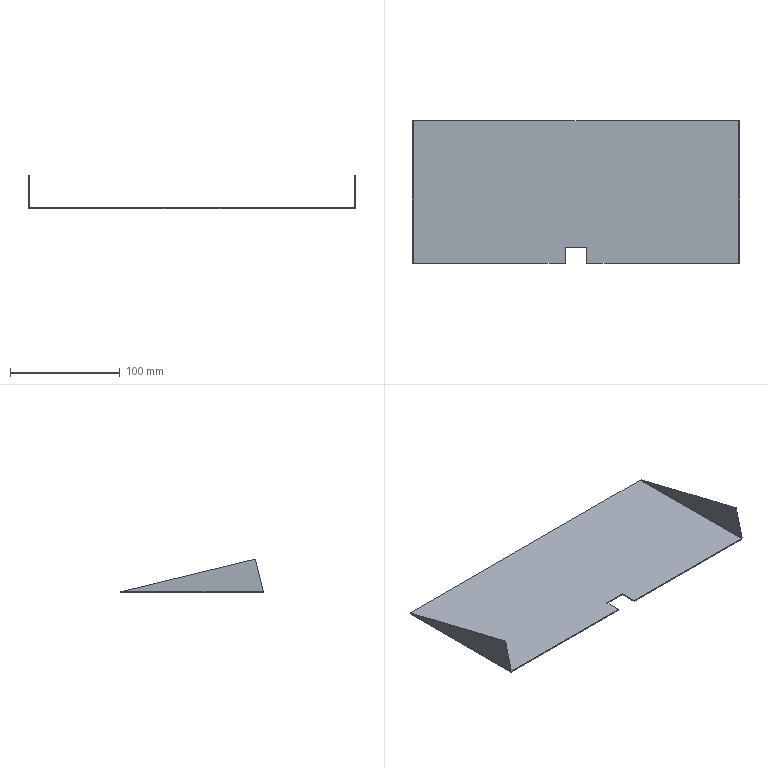Part | SolidWorks | features Cut 1, EdgeFlange 1, FlatPattern 1, MirrorPattern 1, SMBaseFlange 1, SheetMetal 1 | 1 solid | 24 faces | box 299 x 130.5 x 31 mm | volume 42555 mm3 | plane 16 | spline 4 | cylinder 4 | commonest cylinder face diameters 0.4 x2 2.4 x2
STEP:
#1=CARTESIAN_POINT('',(10.,-65.25,-1.));
#2=VERTEX_POINT('',#1);
#3=CARTESIAN_POINT('',(10.,-65.25,0.));
#4=VERTEX_POINT('',#3);
#5=CARTESIAN_POINT('',(10.,-65.25,-1.));
#6=DIRECTION('',(0.,0.,1.));
#7=VECTOR('',#6,1000.);
#8=LINE('',#5,#7);
#9=EDGE_CURVE('',#2,#4,#8,.T.);
#10=ORIENTED_EDGE('',*,*,#9,.F.);
#11=CARTESIAN_POINT('',(148.3,-65.25,-1.));
#12=VERTEX_POINT('',#11);
#13=CARTESIAN_POINT('',(-149.5,-65.25,-1.));
#14=DIRECTION('',(1.,0.,0.));
#15=VECTOR('',#14,1000.);
#16=LINE('',#13,#15);
#17=EDGE_CURVE('',#2,#12,#16,.T.);
#18=ORIENTED_EDGE('',*,*,#17,.T.);
#19=CARTESIAN_POINT('',(148.3,-65.25,0.));
#20=VERTEX_POINT('',#19);
#21=CARTESIAN_POINT('',(148.3,-65.25,0.));
#22=DIRECTION('',(0.,0.,-1.));
#23=VECTOR('',#22,1000.);
#24=LINE('',#21,#23);
#25=EDGE_CURVE('',#20,#12,#24,.T.);
#26=ORIENTED_EDGE('',*,*,#25,.F.);
#27=CARTESIAN_POINT('',(-149.5,-65.25,0.));
#28=DIRECTION('',(1.,0.,0.));
#29=VECTOR('',#28,1000.);
#30=LINE('',#27,#29);
#31=EDGE_CURVE('',#4,#20,#30,.T.);
#32=ORIENTED_EDGE('',*,*,#31,.F.);
#33=EDGE_LOOP('',(#10,#18,#26,#32));
#34=FACE_OUTER_BOUND('',#33,.T.);
#35=CARTESIAN_POINT('',(-149.5,-65.25,-1.));
#36=DIRECTION('',(0.,-1.,0.));
#37=DIRECTION('',(0.,0.,-1.));
#38=AXIS2_PLACEMENT_3D('',#35,#36,#37);
#39=PLANE('',#38);
#40=ADVANCED_FACE('',(#34),#39,.T.);
#41=ORIENTED_EDGE('',*,*,#17,.F.);
#42=CARTESIAN_POINT('',(10.,-50.25,-1.));
#43=VERTEX_POINT('',#42);
#44=CARTESIAN_POINT('',(10.,0.,-1.));
#45=DIRECTION('',(0.,1.,0.));
#46=VECTOR('',#45,1000.);
#47=LINE('',#44,#46);
#48=EDGE_CURVE('',#2,#43,#47,.T.);
#49=ORIENTED_EDGE('',*,*,#48,.T.);
#50=CARTESIAN_POINT('',(-10.,-50.25,-1.));
#51=VERTEX_POINT('',#50);
#52=CARTESIAN_POINT('',(0.,-50.25,-1.));
#53=DIRECTION('',(-1.,0.,0.));
#54=VECTOR('',#53,1000.);
#55=LINE('',#52,#54);
#56=EDGE_CURVE('',#43,#51,#55,.T.);
#57=ORIENTED_EDGE('',*,*,#56,.T.);
#58=CARTESIAN_POINT('',(-10.,-65.25,-1.));
#59=VERTEX_POINT('',#58);
#60=CARTESIAN_POINT('',(-10.,0.,-1.));
#61=DIRECTION('',(0.,-1.,0.));
#62=VECTOR('',#61,1000.);
#63=LINE('',#60,#62);
#64=EDGE_CURVE('',#51,#59,#63,.T.);
#65=ORIENTED_EDGE('',*,*,#64,.T.);
#66=CARTESIAN_POINT('',(-148.3,-65.25,-1.));
#67=VERTEX_POINT('',#66);
#68=CARTESIAN_POINT('',(-149.5,-65.25,-1.));
#69=DIRECTION('',(1.,0.,0.));
#70=VECTOR('',#69,1000.);
#71=LINE('',#68,#70);
#72=EDGE_CURVE('',#67,#59,#71,.T.);
#73=ORIENTED_EDGE('',*,*,#72,.F.);
#74=CARTESIAN_POINT('',(-148.3,65.25,-1.));
#75=VERTEX_POINT('',#74);
#76=CARTESIAN_POINT('',(-148.3,-65.25,-1.));
#77=DIRECTION('',(0.,1.,0.));
#78=VECTOR('',#77,1000.);
#79=LINE('',#76,#78);
#80=EDGE_CURVE('',#67,#75,#79,.T.);
#81=ORIENTED_EDGE('',*,*,#80,.T.);
#82=CARTESIAN_POINT('',(148.3,65.25,-1.));
#83=VERTEX_POINT('',#82);
#84=CARTESIAN_POINT('',(-149.5,65.25,-1.));
#85=DIRECTION('',(-1.,0.,0.));
#86=VECTOR('',#85,1000.);
#87=LINE('',#84,#86);
#88=EDGE_CURVE('',#83,#75,#87,.T.);
#89=ORIENTED_EDGE('',*,*,#88,.F.);
#90=CARTESIAN_POINT('',(148.3,65.25,-1.));
#91=DIRECTION('',(0.,-1.,0.));
#92=VECTOR('',#91,1000.);
#93=LINE('',#90,#92);
#94=EDGE_CURVE('',#83,#12,#93,.T.);
#95=ORIENTED_EDGE('',*,*,#94,.T.);
#96=EDGE_LOOP('',(#41,#49,#57,#65,#73,#81,#89,#95));
#97=FACE_OUTER_BOUND('',#96,.T.);
#98=CARTESIAN_POINT('',(0.,0.,-1.));
#99=DIRECTION('',(0.,0.,1.));
#100=DIRECTION('',(1.,0.,0.));
#101=AXIS2_PLACEMENT_3D('',#98,#99,#100);
#102=PLANE('',#101);
#103=ADVANCED_FACE('',(#97),#102,.F.);
#104=CARTESIAN_POINT('',(10.,-50.25,0.));
#105=VERTEX_POINT('',#104);
#106=CARTESIAN_POINT('',(10.,-50.25,0.));
#107=DIRECTION('',(0.,1.,0.));
#108=VECTOR('',#107,1000.);
#109=LINE('',#106,#108);
#110=EDGE_CURVE('',#4,#105,#109,.T.);
#111=ORIENTED_EDGE('',*,*,#110,.F.);
#112=ORIENTED_EDGE('',*,*,#31,.T.);
#113=CARTESIAN_POINT('',(148.3,65.25,0.));
#114=VERTEX_POINT('',#113);
#115=CARTESIAN_POINT('',(148.3,65.25,0.));
#116=DIRECTION('',(0.,-1.,0.));
#117=VECTOR('',#116,1000.);
#118=LINE('',#115,#117);
#119=EDGE_CURVE('',#114,#20,#118,.T.);
#120=ORIENTED_EDGE('',*,*,#119,.F.);
#121=CARTESIAN_POINT('',(-148.3,65.25,0.));
#122=VERTEX_POINT('',#121);
#123=CARTESIAN_POINT('',(-149.5,65.25,0.));
#124=DIRECTION('',(-1.,0.,0.));
#125=VECTOR('',#124,1000.);
#126=LINE('',#123,#125);
#127=EDGE_CURVE('',#114,#122,#126,.T.);
#128=ORIENTED_EDGE('',*,*,#127,.T.);
#129=CARTESIAN_POINT('',(-148.3,-65.25,0.));
#130=VERTEX_POINT('',#129);
#131=CARTESIAN_POINT('',(-148.3,-65.25,0.));
#132=DIRECTION('',(0.,1.,0.));
#133=VECTOR('',#132,1000.);
#134=LINE('',#131,#133);
#135=EDGE_CURVE('',#130,#122,#134,.T.);
#136=ORIENTED_EDGE('',*,*,#135,.F.);
#137=CARTESIAN_POINT('',(-10.,-65.25,0.));
#138=VERTEX_POINT('',#137);
#139=CARTESIAN_POINT('',(-149.5,-65.25,0.));
#140=DIRECTION('',(1.,0.,0.));
#141=VECTOR('',#140,1000.);
#142=LINE('',#139,#141);
#143=EDGE_CURVE('',#130,#138,#142,.T.);
#144=ORIENTED_EDGE('',*,*,#143,.T.);
#145=CARTESIAN_POINT('',(-10.,-50.25,0.));
#146=VERTEX_POINT('',#145);
#147=CARTESIAN_POINT('',(-10.,-50.25,0.));
#148=DIRECTION('',(0.,-1.,0.));
#149=VECTOR('',#148,1000.);
#150=LINE('',#147,#149);
#151=EDGE_CURVE('',#146,#138,#150,.T.);
#152=ORIENTED_EDGE('',*,*,#151,.F.);
#153=CARTESIAN_POINT('',(-10.,-50.25,0.));
#154=DIRECTION('',(-1.,0.,0.));
#155=VECTOR('',#154,1000.);
#156=LINE('',#153,#155);
#157=EDGE_CURVE('',#105,#146,#156,.T.);
#158=ORIENTED_EDGE('',*,*,#157,.F.);
#159=EDGE_LOOP('',(#111,#112,#120,#128,#136,#144,#152,#158));
#160=FACE_OUTER_BOUND('',#159,.T.);
#161=CARTESIAN_POINT('',(0.,0.,0.));
#162=DIRECTION('',(0.,0.,1.));
#163=DIRECTION('',(1.,0.,0.));
#164=AXIS2_PLACEMENT_3D('',#161,#162,#163);
#165=PLANE('',#164);
#166=ADVANCED_FACE('',(#160),#165,.T.);
#167=ORIENTED_EDGE('',*,*,#127,.F.);
#168=CARTESIAN_POINT('',(148.3,65.25,0.));
#169=DIRECTION('',(0.,0.,-1.));
#170=VECTOR('',#169,1000.);
#171=LINE('',#168,#170);
#172=EDGE_CURVE('',#114,#83,#171,.T.);
#173=ORIENTED_EDGE('',*,*,#172,.T.);
#174=ORIENTED_EDGE('',*,*,#88,.T.);
#175=CARTESIAN_POINT('',(-148.3,65.25,0.));
#176=DIRECTION('',(0.,0.,-1.));
#177=VECTOR('',#176,1000.);
#178=LINE('',#175,#177);
#179=EDGE_CURVE('',#122,#75,#178,.T.);
#180=ORIENTED_EDGE('',*,*,#179,.F.);
#181=EDGE_LOOP('',(#167,#173,#174,#180));
#182=FACE_OUTER_BOUND('',#181,.T.);
#183=CARTESIAN_POINT('',(-149.5,65.25,-1.));
#184=DIRECTION('',(0.,1.,0.));
#185=DIRECTION('',(0.,0.,1.));
#186=AXIS2_PLACEMENT_3D('',#183,#184,#185);
#187=PLANE('',#186);
#188=ADVANCED_FACE('',(#182),#187,.T.);
#189=CARTESIAN_POINT('',(-10.,-65.25,-1.));
#190=DIRECTION('',(0.,0.,-1.));
#191=VECTOR('',#190,1000.);
#192=LINE('',#189,#191);
#193=EDGE_CURVE('',#138,#59,#192,.T.);
#194=ORIENTED_EDGE('',*,*,#193,.F.);
#195=ORIENTED_EDGE('',*,*,#143,.F.);
#196=CARTESIAN_POINT('',(-148.3,-65.25,0.));
#197=DIRECTION('',(0.,0.,-1.));
#198=VECTOR('',#197,1000.);
#199=LINE('',#196,#198);
#200=EDGE_CURVE('',#130,#67,#199,.T.);
#201=ORIENTED_EDGE('',*,*,#200,.T.);
#202=ORIENTED_EDGE('',*,*,#72,.T.);
#203=EDGE_LOOP('',(#194,#195,#201,#202));
#204=FACE_OUTER_BOUND('',#203,.T.);
#205=CARTESIAN_POINT('',(-149.5,-65.25,-1.));
#206=DIRECTION('',(0.,-1.,0.));
#207=DIRECTION('',(0.,0.,-1.));
#208=AXIS2_PLACEMENT_3D('',#205,#206,#207);
#209=PLANE('',#208);
#210=ADVANCED_FACE('',(#204),#209,.T.);
#211=CARTESIAN_POINT('',(-148.5,64.429,0.2));
#212=VERTEX_POINT('',#211);
#213=CARTESIAN_POINT('',(-149.5,64.429,0.2));
#214=VERTEX_POINT('',#213);
#215=CARTESIAN_POINT('',(-149.5,64.429,0.2));
#216=DIRECTION('',(-1.,0.,0.));
#217=VECTOR('',#216,1000.);
#218=LINE('',#215,#217);
#219=EDGE_CURVE('',#212,#214,#218,.T.);
#220=ORIENTED_EDGE('',*,*,#219,.F.);
#221=CARTESIAN_POINT('',(-148.3,65.25,0.));
#222=CARTESIAN_POINT('',(-148.352,65.113,0.));
#223=CARTESIAN_POINT('',(-148.404,64.976,0.02155));
#224=CARTESIAN_POINT('',(-148.478,64.702,0.0956));
#225=CARTESIAN_POINT('',(-148.5,64.566,0.1476));
#226=CARTESIAN_POINT('',(-148.5,64.429,0.2));
#227=B_SPLINE_CURVE_WITH_KNOTS('',3,(#221,#222,#223,#224,#225,#226),.UNSPECIFIED.,.F.,.F.,(4,2,4),(0.,0.5,1.),.UNSPECIFIED.);
#228=EDGE_CURVE('',#122,#212,#227,.T.);
#229=ORIENTED_EDGE('',*,*,#228,.F.);
#230=ORIENTED_EDGE('',*,*,#179,.T.);
#231=CARTESIAN_POINT('',(-148.3,65.25,-1.));
#232=CARTESIAN_POINT('',(-148.459,65.181,-1.));
#233=CARTESIAN_POINT('',(-148.612,65.114,-0.9695));
#234=CARTESIAN_POINT('',(-148.905,64.976,-0.8483));
#235=CARTESIAN_POINT('',(-149.036,64.908,-0.7606));
#236=CARTESIAN_POINT('',(-149.26,64.771,-0.5372));
#237=CARTESIAN_POINT('',(-149.348,64.703,-0.4051));
#238=CARTESIAN_POINT('',(-149.469,64.566,-0.1141));
#239=CARTESIAN_POINT('',(-149.5,64.498,0.04143));
#240=CARTESIAN_POINT('',(-149.5,64.429,0.2));
#241=B_SPLINE_CURVE_WITH_KNOTS('',3,(#231,#232,#233,#234,#235,#236,#237,#238,#239,#240),.UNSPECIFIED.,.F.,.F.,(4,2,2,2,4),(0.,0.0005105,0.001021,0.001532,0.002042),.UNSPECIFIED.);
#242=EDGE_CURVE('',#75,#214,#241,.T.);
#243=ORIENTED_EDGE('',*,*,#242,.T.);
#244=EDGE_LOOP('',(#220,#229,#230,#243));
#245=FACE_OUTER_BOUND('',#244,.T.);
#246=CARTESIAN_POINT('',(-148.3,65.25,-1.01));
#247=CARTESIAN_POINT('',(-148.458,65.182,-1.01));
#248=CARTESIAN_POINT('',(-148.617,65.113,-0.9785));
#249=CARTESIAN_POINT('',(-148.909,64.976,-0.8573));
#250=CARTESIAN_POINT('',(-149.044,64.908,-0.7676));
#251=CARTESIAN_POINT('',(-149.268,64.771,-0.5436));
#252=CARTESIAN_POINT('',(-149.357,64.702,-0.4094));
#253=CARTESIAN_POINT('',(-149.479,64.566,-0.1167));
#254=CARTESIAN_POINT('',(-149.51,64.497,0.04159));
#255=CARTESIAN_POINT('',(-149.51,64.429,0.2));
#256=CARTESIAN_POINT('',(-148.3,65.25,-1.));
#257=CARTESIAN_POINT('',(-148.457,65.182,-1.));
#258=CARTESIAN_POINT('',(-148.614,65.113,-0.9688));
#259=CARTESIAN_POINT('',(-148.904,64.976,-0.8485));
#260=CARTESIAN_POINT('',(-149.037,64.908,-0.7596));
#261=CARTESIAN_POINT('',(-149.26,64.771,-0.5375));
#262=CARTESIAN_POINT('',(-149.349,64.702,-0.4043));
#263=CARTESIAN_POINT('',(-149.469,64.566,-0.1141));
#264=CARTESIAN_POINT('',(-149.5,64.497,0.0429));
#265=CARTESIAN_POINT('',(-149.5,64.429,0.2));
#266=CARTESIAN_POINT('',(-148.3,65.25,0.));
#267=CARTESIAN_POINT('',(-148.326,65.182,0.));
#268=CARTESIAN_POINT('',(-148.352,65.113,0.005205));
#269=CARTESIAN_POINT('',(-148.401,64.976,0.02524));
#270=CARTESIAN_POINT('',(-148.423,64.908,0.04007));
#271=CARTESIAN_POINT('',(-148.46,64.771,0.07709));
#272=CARTESIAN_POINT('',(-148.475,64.702,0.09928));
#273=CARTESIAN_POINT('',(-148.495,64.566,0.1477));
#274=CARTESIAN_POINT('',(-148.5,64.497,0.1738));
#275=CARTESIAN_POINT('',(-148.5,64.429,0.2));
#276=CARTESIAN_POINT('',(-148.3,65.25,0.0101));
#277=CARTESIAN_POINT('',(-148.325,65.182,0.0101));
#278=CARTESIAN_POINT('',(-148.35,65.113,0.01504));
#279=CARTESIAN_POINT('',(-148.396,64.976,0.03407));
#280=CARTESIAN_POINT('',(-148.417,64.908,0.04814));
#281=CARTESIAN_POINT('',(-148.452,64.771,0.0833));
#282=CARTESIAN_POINT('',(-148.466,64.702,0.1044));
#283=CARTESIAN_POINT('',(-148.485,64.566,0.1503));
#284=CARTESIAN_POINT('',(-148.49,64.497,0.1751));
#285=CARTESIAN_POINT('',(-148.49,64.429,0.2));
#286=B_SPLINE_SURFACE_WITH_KNOTS('',1,3,((#246,#247,#248,#249,#250,#251,#252,#253,#254,#255),(#256,#257,#258,#259,#260,#261,#262,#263,#264,#265),(#266,#267,#268,#269,#270,#271,#272,#273,#274,#275),(#276,#277,#278,#279,#280,#281,#282,#283,#284,#285)),.UNSPECIFIED.,.F.,.F.,.F.,(2,1,1,2),(4,2,2,2,4),(-0.01,0.,1.,1.01),(0.,0.25,0.5,0.75,1.),.UNSPECIFIED.);
#287=ADVANCED_FACE('',(#245),#286,.F.);
#288=CARTESIAN_POINT('',(-148.5,-65.201,0.2));
#289=VERTEX_POINT('',#288);
#290=CARTESIAN_POINT('',(-148.5,-65.201,0.2));
#291=CARTESIAN_POINT('',(-148.5,-65.209,0.1476));
#292=CARTESIAN_POINT('',(-148.478,-65.218,0.0956));
#293=CARTESIAN_POINT('',(-148.404,-65.234,0.02155));
#294=CARTESIAN_POINT('',(-148.352,-65.242,0.));
#295=CARTESIAN_POINT('',(-148.3,-65.25,0.));
#296=B_SPLINE_CURVE_WITH_KNOTS('',3,(#290,#291,#292,#293,#294,#295),.UNSPECIFIED.,.F.,.F.,(4,2,4),(0.,0.5,1.),.UNSPECIFIED.);
#297=EDGE_CURVE('',#289,#130,#296,.T.);
#298=ORIENTED_EDGE('',*,*,#297,.F.);
#299=CARTESIAN_POINT('',(-149.5,-65.201,0.2));
#300=VERTEX_POINT('',#299);
#301=CARTESIAN_POINT('',(-148.5,-65.201,0.2));
#302=DIRECTION('',(-1.,0.,0.));
#303=VECTOR('',#302,1000.);
#304=LINE('',#301,#303);
#305=EDGE_CURVE('',#289,#300,#304,.T.);
#306=ORIENTED_EDGE('',*,*,#305,.T.);
#307=CARTESIAN_POINT('',(-149.5,-65.201,0.2));
#308=CARTESIAN_POINT('',(-149.5,-65.205,0.04292));
#309=CARTESIAN_POINT('',(-149.469,-65.209,-0.1141));
#310=CARTESIAN_POINT('',(-149.349,-65.218,-0.4043));
#311=CARTESIAN_POINT('',(-149.26,-65.222,-0.5375));
#312=CARTESIAN_POINT('',(-149.037,-65.23,-0.7596));
#313=CARTESIAN_POINT('',(-148.904,-65.234,-0.8485));
#314=CARTESIAN_POINT('',(-148.614,-65.242,-0.9688));
#315=CARTESIAN_POINT('',(-148.457,-65.246,-1.));
#316=CARTESIAN_POINT('',(-148.3,-65.25,-1.));
#317=B_SPLINE_CURVE_WITH_KNOTS('',3,(#307,#308,#309,#310,#311,#312,#313,#314,#315,#316),.UNSPECIFIED.,.F.,.F.,(4,2,2,2,4),(0.,0.25,0.5,0.75,1.),.UNSPECIFIED.);
#318=EDGE_CURVE('',#300,#67,#317,.T.);
#319=ORIENTED_EDGE('',*,*,#318,.T.);
#320=ORIENTED_EDGE('',*,*,#200,.F.);
#321=EDGE_LOOP('',(#298,#306,#319,#320));
#322=FACE_OUTER_BOUND('',#321,.T.);
#323=CARTESIAN_POINT('',(-149.51,-65.201,0.2));
#324=CARTESIAN_POINT('',(-149.51,-65.205,0.04158));
#325=CARTESIAN_POINT('',(-149.479,-65.209,-0.1167));
#326=CARTESIAN_POINT('',(-149.357,-65.218,-0.4094));
#327=CARTESIAN_POINT('',(-149.268,-65.222,-0.5436));
#328=CARTESIAN_POINT('',(-149.044,-65.23,-0.7676));
#329=CARTESIAN_POINT('',(-148.909,-65.234,-0.8573));
#330=CARTESIAN_POINT('',(-148.617,-65.242,-0.9785));
#331=CARTESIAN_POINT('',(-148.458,-65.246,-1.01));
#332=CARTESIAN_POINT('',(-148.3,-65.25,-1.01));
#333=CARTESIAN_POINT('',(-149.5,-65.201,0.2));
#334=CARTESIAN_POINT('',(-149.5,-65.205,0.04289));
#335=CARTESIAN_POINT('',(-149.469,-65.209,-0.1141));
#336=CARTESIAN_POINT('',(-149.349,-65.218,-0.4043));
#337=CARTESIAN_POINT('',(-149.26,-65.222,-0.5375));
#338=CARTESIAN_POINT('',(-149.037,-65.23,-0.7596));
#339=CARTESIAN_POINT('',(-148.904,-65.234,-0.8485));
#340=CARTESIAN_POINT('',(-148.614,-65.242,-0.9688));
#341=CARTESIAN_POINT('',(-148.457,-65.246,-1.));
#342=CARTESIAN_POINT('',(-148.3,-65.25,-1.));
#343=CARTESIAN_POINT('',(-148.5,-65.201,0.2));
#344=CARTESIAN_POINT('',(-148.5,-65.205,0.1738));
#345=CARTESIAN_POINT('',(-148.495,-65.209,0.1477));
#346=CARTESIAN_POINT('',(-148.475,-65.218,0.09928));
#347=CARTESIAN_POINT('',(-148.46,-65.222,0.07709));
#348=CARTESIAN_POINT('',(-148.423,-65.23,0.04007));
#349=CARTESIAN_POINT('',(-148.401,-65.234,0.02524));
#350=CARTESIAN_POINT('',(-148.352,-65.242,0.005205));
#351=CARTESIAN_POINT('',(-148.326,-65.246,0.));
#352=CARTESIAN_POINT('',(-148.3,-65.25,0.));
#353=CARTESIAN_POINT('',(-148.49,-65.201,0.2));
#354=CARTESIAN_POINT('',(-148.49,-65.205,0.1751));
#355=CARTESIAN_POINT('',(-148.485,-65.209,0.1503));
#356=CARTESIAN_POINT('',(-148.466,-65.218,0.1044));
#357=CARTESIAN_POINT('',(-148.452,-65.222,0.0833));
#358=CARTESIAN_POINT('',(-148.417,-65.23,0.04814));
#359=CARTESIAN_POINT('',(-148.396,-65.234,0.03407));
#360=CARTESIAN_POINT('',(-148.35,-65.242,0.01504));
#361=CARTESIAN_POINT('',(-148.325,-65.246,0.0101));
#362=CARTESIAN_POINT('',(-148.3,-65.25,0.0101));
#363=B_SPLINE_SURFACE_WITH_KNOTS('',1,3,((#323,#324,#325,#326,#327,#328,#329,#330,#331,#332),(#333,#334,#335,#336,#337,#338,#339,#340,#341,#342),(#343,#344,#345,#346,#347,#348,#349,#350,#351,#352),(#353,#354,#355,#356,#357,#358,#359,#360,#361,#362)),.UNSPECIFIED.,.F.,.F.,.F.,(2,1,1,2),(4,2,2,2,4),(-0.01,0.,1.,1.01),(0.,0.25,0.5,0.75,1.),.UNSPECIFIED.);
#364=ADVANCED_FACE('',(#322),#363,.F.);
#365=ORIENTED_EDGE('',*,*,#80,.F.);
#366=ORIENTED_EDGE('',*,*,#318,.F.);
#367=CARTESIAN_POINT('',(-149.5,64.429,0.2));
#368=DIRECTION('',(0.,1.,0.));
#369=VECTOR('',#368,1000.);
#370=LINE('',#367,#369);
#371=EDGE_CURVE('',#300,#214,#370,.T.);
#372=ORIENTED_EDGE('',*,*,#371,.T.);
#373=ORIENTED_EDGE('',*,*,#242,.F.);
#374=EDGE_LOOP('',(#365,#366,#372,#373));
#375=FACE_OUTER_BOUND('',#374,.T.);
#376=CARTESIAN_POINT('',(-148.3,-65.25,0.2));
#377=DIRECTION('',(0.,-1.,0.));
#378=DIRECTION('',(-1.,0.,0.));
#379=AXIS2_PLACEMENT_3D('',#376,#377,#378);
#380=CYLINDRICAL_SURFACE('',#379,1.2);
#381=ADVANCED_FACE('',(#375),#380,.T.);
#382=ORIENTED_EDGE('',*,*,#135,.T.);
#383=ORIENTED_EDGE('',*,*,#228,.T.);
#384=CARTESIAN_POINT('',(-148.5,64.429,0.2));
#385=DIRECTION('',(0.,-1.,0.));
#386=VECTOR('',#385,1000.);
#387=LINE('',#384,#386);
#388=EDGE_CURVE('',#212,#289,#387,.T.);
#389=ORIENTED_EDGE('',*,*,#388,.T.);
#390=ORIENTED_EDGE('',*,*,#297,.T.);
#391=EDGE_LOOP('',(#382,#383,#389,#390));
#392=FACE_OUTER_BOUND('',#391,.T.);
#393=CARTESIAN_POINT('',(-148.3,-65.25,0.2));
#394=DIRECTION('',(0.,-1.,0.));
#395=DIRECTION('',(-1.,0.,0.));
#396=AXIS2_PLACEMENT_3D('',#393,#394,#395);
#397=CYLINDRICAL_SURFACE('',#396,0.2);
#398=ADVANCED_FACE('',(#392),#397,.F.);
#399=ORIENTED_EDGE('',*,*,#219,.T.);
#400=CARTESIAN_POINT('',(-149.5,-57.944,30.));
#401=VERTEX_POINT('',#400);
#402=CARTESIAN_POINT('',(-149.5,3.653,15.));
#403=DIRECTION('',(0.,0.9716,-0.2366));
#404=VECTOR('',#403,1000.);
#405=LINE('',#402,#404);
#406=EDGE_CURVE('',#401,#214,#405,.T.);
#407=ORIENTED_EDGE('',*,*,#406,.F.);
#408=CARTESIAN_POINT('',(-148.5,-57.944,30.));
#409=VERTEX_POINT('',#408);
#410=CARTESIAN_POINT('',(-149.5,-57.944,30.));
#411=DIRECTION('',(1.,0.,0.));
#412=VECTOR('',#411,1000.);
#413=LINE('',#410,#412);
#414=EDGE_CURVE('',#401,#409,#413,.T.);
#415=ORIENTED_EDGE('',*,*,#414,.T.);
#416=CARTESIAN_POINT('',(-148.5,-57.944,30.));
#417=DIRECTION('',(0.,0.9716,-0.2366));
#418=VECTOR('',#417,1000.);
#419=LINE('',#416,#418);
#420=EDGE_CURVE('',#409,#212,#419,.T.);
#421=ORIENTED_EDGE('',*,*,#420,.T.);
#422=EDGE_LOOP('',(#399,#407,#415,#421));
#423=FACE_OUTER_BOUND('',#422,.T.);
#424=CARTESIAN_POINT('',(-149.5,-57.944,30.));
#425=DIRECTION('',(0.,-0.2366,-0.9716));
#426=DIRECTION('',(0.,0.9716,-0.2366));
#427=AXIS2_PLACEMENT_3D('',#424,#425,#426);
#428=PLANE('',#427);
#429=ADVANCED_FACE('',(#423),#428,.F.);
#430=ORIENTED_EDGE('',*,*,#305,.F.);
#431=CARTESIAN_POINT('',(-148.5,-65.25,0.));
#432=DIRECTION('',(0.,0.2366,0.9716));
#433=VECTOR('',#432,1000.);
#434=LINE('',#431,#433);
#435=EDGE_CURVE('',#289,#409,#434,.T.);
#436=ORIENTED_EDGE('',*,*,#435,.T.);
#437=ORIENTED_EDGE('',*,*,#414,.F.);
#438=CARTESIAN_POINT('',(-149.5,-61.597,15.));
#439=DIRECTION('',(0.,0.2366,0.9716));
#440=VECTOR('',#439,1000.);
#441=LINE('',#438,#440);
#442=EDGE_CURVE('',#300,#401,#441,.T.);
#443=ORIENTED_EDGE('',*,*,#442,.F.);
#444=EDGE_LOOP('',(#430,#436,#437,#443));
#445=FACE_OUTER_BOUND('',#444,.T.);
#446=CARTESIAN_POINT('',(-149.5,-65.25,0.));
#447=DIRECTION('',(0.,0.9716,-0.2366));
#448=DIRECTION('',(0.,0.2366,0.9716));
#449=AXIS2_PLACEMENT_3D('',#446,#447,#448);
#450=PLANE('',#449);
#451=ADVANCED_FACE('',(#445),#450,.F.);
#452=ORIENTED_EDGE('',*,*,#371,.F.);
#453=ORIENTED_EDGE('',*,*,#442,.T.);
#454=ORIENTED_EDGE('',*,*,#406,.T.);
#455=EDGE_LOOP('',(#452,#453,#454));
#456=FACE_OUTER_BOUND('',#455,.T.);
#457=CARTESIAN_POINT('',(-149.5,0.,0.));
#458=DIRECTION('',(1.,0.,0.));
#459=DIRECTION('',(0.,0.,-1.));
#460=AXIS2_PLACEMENT_3D('',#457,#458,#459);
#461=PLANE('',#460);
#462=ADVANCED_FACE('',(#456),#461,.F.);
#463=ORIENTED_EDGE('',*,*,#435,.F.);
#464=ORIENTED_EDGE('',*,*,#388,.F.);
#465=ORIENTED_EDGE('',*,*,#420,.F.);
#466=EDGE_LOOP('',(#463,#464,#465));
#467=FACE_OUTER_BOUND('',#466,.T.);
#468=CARTESIAN_POINT('',(-148.5,0.,0.));
#469=DIRECTION('',(1.,0.,0.));
#470=DIRECTION('',(0.,0.,-1.));
#471=AXIS2_PLACEMENT_3D('',#468,#469,#470);
#472=PLANE('',#471);
#473=ADVANCED_FACE('',(#467),#472,.T.);
#474=CARTESIAN_POINT('',(148.5,-65.201,0.2));
#475=VERTEX_POINT('',#474);
#476=CARTESIAN_POINT('',(149.5,-65.201,0.2));
#477=VERTEX_POINT('',#476);
#478=CARTESIAN_POINT('',(149.5,-65.201,0.2));
#479=DIRECTION('',(1.,0.,0.));
#480=VECTOR('',#479,1000.);
#481=LINE('',#478,#480);
#482=EDGE_CURVE('',#475,#477,#481,.T.);
#483=ORIENTED_EDGE('',*,*,#482,.F.);
#484=CARTESIAN_POINT('',(148.3,-65.25,0.));
#485=CARTESIAN_POINT('',(148.352,-65.242,0.));
#486=CARTESIAN_POINT('',(148.404,-65.234,0.02155));
#487=CARTESIAN_POINT('',(148.478,-65.218,0.0956));
#488=CARTESIAN_POINT('',(148.5,-65.209,0.1476));
#489=CARTESIAN_POINT('',(148.5,-65.201,0.2));
#490=B_SPLINE_CURVE_WITH_KNOTS('',3,(#484,#485,#486,#487,#488,#489),.UNSPECIFIED.,.F.,.F.,(4,2,4),(0.,0.5,1.),.UNSPECIFIED.);
#491=EDGE_CURVE('',#20,#475,#490,.T.);
#492=ORIENTED_EDGE('',*,*,#491,.F.);
#493=ORIENTED_EDGE('',*,*,#25,.T.);
#494=CARTESIAN_POINT('',(148.3,-65.25,-1.));
#495=CARTESIAN_POINT('',(148.457,-65.246,-1.));
#496=CARTESIAN_POINT('',(148.614,-65.242,-0.9688));
#497=CARTESIAN_POINT('',(148.904,-65.234,-0.8485));
#498=CARTESIAN_POINT('',(149.037,-65.23,-0.7596));
#499=CARTESIAN_POINT('',(149.26,-65.222,-0.5375));
#500=CARTESIAN_POINT('',(149.349,-65.218,-0.4043));
#501=CARTESIAN_POINT('',(149.469,-65.209,-0.1141));
#502=CARTESIAN_POINT('',(149.5,-65.205,0.04292));
#503=CARTESIAN_POINT('',(149.5,-65.201,0.2));
#504=B_SPLINE_CURVE_WITH_KNOTS('',3,(#494,#495,#496,#497,#498,#499,#500,#501,#502,#503),.UNSPECIFIED.,.F.,.F.,(4,2,2,2,4),(0.,0.25,0.5,0.75,1.),.UNSPECIFIED.);
#505=EDGE_CURVE('',#12,#477,#504,.T.);
#506=ORIENTED_EDGE('',*,*,#505,.T.);
#507=EDGE_LOOP('',(#483,#492,#493,#506));
#508=FACE_OUTER_BOUND('',#507,.T.);
#509=CARTESIAN_POINT('',(148.3,-65.25,-1.01));
#510=CARTESIAN_POINT('',(148.458,-65.246,-1.01));
#511=CARTESIAN_POINT('',(148.617,-65.242,-0.9785));
#512=CARTESIAN_POINT('',(148.909,-65.234,-0.8573));
#513=CARTESIAN_POINT('',(149.044,-65.23,-0.7676));
#514=CARTESIAN_POINT('',(149.268,-65.222,-0.5436));
#515=CARTESIAN_POINT('',(149.357,-65.218,-0.4094));
#516=CARTESIAN_POINT('',(149.479,-65.209,-0.1167));
#517=CARTESIAN_POINT('',(149.51,-65.205,0.04158));
#518=CARTESIAN_POINT('',(149.51,-65.201,0.2));
#519=CARTESIAN_POINT('',(148.3,-65.25,-1.));
#520=CARTESIAN_POINT('',(148.457,-65.246,-1.));
#521=CARTESIAN_POINT('',(148.614,-65.242,-0.9688));
#522=CARTESIAN_POINT('',(148.904,-65.234,-0.8485));
#523=CARTESIAN_POINT('',(149.037,-65.23,-0.7596));
#524=CARTESIAN_POINT('',(149.26,-65.222,-0.5375));
#525=CARTESIAN_POINT('',(149.349,-65.218,-0.4043));
#526=CARTESIAN_POINT('',(149.469,-65.209,-0.1141));
#527=CARTESIAN_POINT('',(149.5,-65.205,0.04289));
#528=CARTESIAN_POINT('',(149.5,-65.201,0.2));
#529=CARTESIAN_POINT('',(148.3,-65.25,0.));
#530=CARTESIAN_POINT('',(148.326,-65.246,0.));
#531=CARTESIAN_POINT('',(148.352,-65.242,0.005205));
#532=CARTESIAN_POINT('',(148.401,-65.234,0.02524));
#533=CARTESIAN_POINT('',(148.423,-65.23,0.04007));
#534=CARTESIAN_POINT('',(148.46,-65.222,0.07709));
#535=CARTESIAN_POINT('',(148.475,-65.218,0.09928));
#536=CARTESIAN_POINT('',(148.495,-65.209,0.1477));
#537=CARTESIAN_POINT('',(148.5,-65.205,0.1738));
#538=CARTESIAN_POINT('',(148.5,-65.201,0.2));
#539=CARTESIAN_POINT('',(148.3,-65.25,0.0101));
#540=CARTESIAN_POINT('',(148.325,-65.246,0.0101));
#541=CARTESIAN_POINT('',(148.35,-65.242,0.01504));
#542=CARTESIAN_POINT('',(148.396,-65.234,0.03407));
#543=CARTESIAN_POINT('',(148.417,-65.23,0.04814));
#544=CARTESIAN_POINT('',(148.452,-65.222,0.0833));
#545=CARTESIAN_POINT('',(148.466,-65.218,0.1044));
#546=CARTESIAN_POINT('',(148.485,-65.209,0.1503));
#547=CARTESIAN_POINT('',(148.49,-65.205,0.1751));
#548=CARTESIAN_POINT('',(148.49,-65.201,0.2));
#549=B_SPLINE_SURFACE_WITH_KNOTS('',1,3,((#509,#510,#511,#512,#513,#514,#515,#516,#517,#518),(#519,#520,#521,#522,#523,#524,#525,#526,#527,#528),(#529,#530,#531,#532,#533,#534,#535,#536,#537,#538),(#539,#540,#541,#542,#543,#544,#545,#546,#547,#548)),.UNSPECIFIED.,.F.,.F.,.F.,(2,1,1,2),(4,2,2,2,4),(-0.01,0.,1.,1.01),(0.,0.25,0.5,0.75,1.),.UNSPECIFIED.);
#550=ADVANCED_FACE('',(#508),#549,.F.);
#551=CARTESIAN_POINT('',(148.5,64.429,0.2));
#552=VERTEX_POINT('',#551);
#553=CARTESIAN_POINT('',(148.5,64.429,0.2));
#554=CARTESIAN_POINT('',(148.5,64.566,0.1476));
#555=CARTESIAN_POINT('',(148.478,64.702,0.0956));
#556=CARTESIAN_POINT('',(148.404,64.976,0.02155));
#557=CARTESIAN_POINT('',(148.352,65.113,0.));
#558=CARTESIAN_POINT('',(148.3,65.25,0.));
#559=B_SPLINE_CURVE_WITH_KNOTS('',3,(#553,#554,#555,#556,#557,#558),.UNSPECIFIED.,.F.,.F.,(4,2,4),(0.,0.5,1.),.UNSPECIFIED.);
#560=EDGE_CURVE('',#552,#114,#559,.T.);
#561=ORIENTED_EDGE('',*,*,#560,.F.);
#562=CARTESIAN_POINT('',(149.5,64.429,0.2));
#563=VERTEX_POINT('',#562);
#564=CARTESIAN_POINT('',(148.5,64.429,0.2));
#565=DIRECTION('',(1.,0.,0.));
#566=VECTOR('',#565,1000.);
#567=LINE('',#564,#566);
#568=EDGE_CURVE('',#552,#563,#567,.T.);
#569=ORIENTED_EDGE('',*,*,#568,.T.);
#570=CARTESIAN_POINT('',(149.5,64.429,0.2));
#571=CARTESIAN_POINT('',(149.5,64.498,0.04143));
#572=CARTESIAN_POINT('',(149.47,64.565,-0.1121));
#573=CARTESIAN_POINT('',(149.348,64.703,-0.4051));
#574=CARTESIAN_POINT('',(149.261,64.77,-0.5364));
#575=CARTESIAN_POINT('',(149.037,64.908,-0.76));
#576=CARTESIAN_POINT('',(148.905,64.976,-0.8482));
#577=CARTESIAN_POINT('',(148.614,65.113,-0.9688));
#578=CARTESIAN_POINT('',(148.459,65.181,-1.));
#579=CARTESIAN_POINT('',(148.3,65.25,-1.));
#580=B_SPLINE_CURVE_WITH_KNOTS('',3,(#570,#571,#572,#573,#574,#575,#576,#577,#578,#579),.UNSPECIFIED.,.F.,.F.,(4,2,2,2,4),(0.,0.0005105,0.001021,0.001532,0.002042),.UNSPECIFIED.);
#581=EDGE_CURVE('',#563,#83,#580,.T.);
#582=ORIENTED_EDGE('',*,*,#581,.T.);
#583=ORIENTED_EDGE('',*,*,#172,.F.);
#584=EDGE_LOOP('',(#561,#569,#582,#583));
#585=FACE_OUTER_BOUND('',#584,.T.);
#586=CARTESIAN_POINT('',(149.51,64.429,0.2));
#587=CARTESIAN_POINT('',(149.51,64.497,0.04159));
#588=CARTESIAN_POINT('',(149.479,64.566,-0.1167));
#589=CARTESIAN_POINT('',(149.357,64.702,-0.4094));
#590=CARTESIAN_POINT('',(149.268,64.771,-0.5436));
#591=CARTESIAN_POINT('',(149.044,64.908,-0.7676));
#592=CARTESIAN_POINT('',(148.909,64.976,-0.8573));
#593=CARTESIAN_POINT('',(148.617,65.113,-0.9785));
#594=CARTESIAN_POINT('',(148.458,65.182,-1.01));
#595=CARTESIAN_POINT('',(148.3,65.25,-1.01));
#596=CARTESIAN_POINT('',(149.5,64.429,0.2));
#597=CARTESIAN_POINT('',(149.5,64.497,0.0429));
#598=CARTESIAN_POINT('',(149.469,64.566,-0.1141));
#599=CARTESIAN_POINT('',(149.349,64.702,-0.4043));
#600=CARTESIAN_POINT('',(149.26,64.771,-0.5375));
#601=CARTESIAN_POINT('',(149.037,64.908,-0.7596));
#602=CARTESIAN_POINT('',(148.904,64.976,-0.8485));
#603=CARTESIAN_POINT('',(148.614,65.113,-0.9688));
#604=CARTESIAN_POINT('',(148.457,65.182,-1.));
#605=CARTESIAN_POINT('',(148.3,65.25,-1.));
#606=CARTESIAN_POINT('',(148.5,64.429,0.2));
#607=CARTESIAN_POINT('',(148.5,64.497,0.1738));
#608=CARTESIAN_POINT('',(148.495,64.566,0.1477));
#609=CARTESIAN_POINT('',(148.475,64.702,0.09928));
#610=CARTESIAN_POINT('',(148.46,64.771,0.07709));
#611=CARTESIAN_POINT('',(148.423,64.908,0.04007));
#612=CARTESIAN_POINT('',(148.401,64.976,0.02524));
#613=CARTESIAN_POINT('',(148.352,65.113,0.005205));
#614=CARTESIAN_POINT('',(148.326,65.182,0.));
#615=CARTESIAN_POINT('',(148.3,65.25,0.));
#616=CARTESIAN_POINT('',(148.49,64.429,0.2));
#617=CARTESIAN_POINT('',(148.49,64.497,0.1751));
#618=CARTESIAN_POINT('',(148.485,64.566,0.1503));
#619=CARTESIAN_POINT('',(148.466,64.702,0.1044));
#620=CARTESIAN_POINT('',(148.452,64.771,0.0833));
#621=CARTESIAN_POINT('',(148.417,64.908,0.04814));
#622=CARTESIAN_POINT('',(148.396,64.976,0.03407));
#623=CARTESIAN_POINT('',(148.35,65.113,0.01504));
#624=CARTESIAN_POINT('',(148.325,65.182,0.0101));
#625=CARTESIAN_POINT('',(148.3,65.25,0.0101));
#626=B_SPLINE_SURFACE_WITH_KNOTS('',1,3,((#586,#587,#588,#589,#590,#591,#592,#593,#594,#595),(#596,#597,#598,#599,#600,#601,#602,#603,#604,#605),(#606,#607,#608,#609,#610,#611,#612,#613,#614,#615),(#616,#617,#618,#619,#620,#621,#622,#623,#624,#625)),.UNSPECIFIED.,.F.,.F.,.F.,(2,1,1,2),(4,2,2,2,4),(-0.01,0.,1.,1.01),(0.,0.25,0.5,0.75,1.),.UNSPECIFIED.);
#627=ADVANCED_FACE('',(#585),#626,.F.);
#628=ORIENTED_EDGE('',*,*,#94,.F.);
#629=ORIENTED_EDGE('',*,*,#581,.F.);
#630=CARTESIAN_POINT('',(149.5,-65.201,0.2));
#631=DIRECTION('',(0.,-1.,0.));
#632=VECTOR('',#631,1000.);
#633=LINE('',#630,#632);
#634=EDGE_CURVE('',#563,#477,#633,.T.);
#635=ORIENTED_EDGE('',*,*,#634,.T.);
#636=ORIENTED_EDGE('',*,*,#505,.F.);
#637=EDGE_LOOP('',(#628,#629,#635,#636));
#638=FACE_OUTER_BOUND('',#637,.T.);
#639=CARTESIAN_POINT('',(148.3,65.25,0.2));
#640=DIRECTION('',(0.,1.,0.));
#641=DIRECTION('',(1.,0.,0.));
#642=AXIS2_PLACEMENT_3D('',#639,#640,#641);
#643=CYLINDRICAL_SURFACE('',#642,1.2);
#644=ADVANCED_FACE('',(#638),#643,.T.);
#645=ORIENTED_EDGE('',*,*,#119,.T.);
#646=ORIENTED_EDGE('',*,*,#491,.T.);
#647=CARTESIAN_POINT('',(148.5,-65.201,0.2));
#648=DIRECTION('',(0.,1.,0.));
#649=VECTOR('',#648,1000.);
#650=LINE('',#647,#649);
#651=EDGE_CURVE('',#475,#552,#650,.T.);
#652=ORIENTED_EDGE('',*,*,#651,.T.);
#653=ORIENTED_EDGE('',*,*,#560,.T.);
#654=EDGE_LOOP('',(#645,#646,#652,#653));
#655=FACE_OUTER_BOUND('',#654,.T.);
#656=CARTESIAN_POINT('',(148.3,65.25,0.2));
#657=DIRECTION('',(0.,1.,0.));
#658=DIRECTION('',(1.,0.,0.));
#659=AXIS2_PLACEMENT_3D('',#656,#657,#658);
#660=CYLINDRICAL_SURFACE('',#659,0.2);
#661=ADVANCED_FACE('',(#655),#660,.F.);
#662=CARTESIAN_POINT('',(149.5,-57.944,30.));
#663=VERTEX_POINT('',#662);
#664=CARTESIAN_POINT('',(149.5,-57.944,30.));
#665=DIRECTION('',(0.,0.9716,-0.2366));
#666=VECTOR('',#665,1000.);
#667=LINE('',#664,#666);
#668=EDGE_CURVE('',#663,#563,#667,.T.);
#669=ORIENTED_EDGE('',*,*,#668,.T.);
#670=ORIENTED_EDGE('',*,*,#568,.F.);
#671=CARTESIAN_POINT('',(148.5,-57.944,30.));
#672=VERTEX_POINT('',#671);
#673=CARTESIAN_POINT('',(148.5,3.653,15.));
#674=DIRECTION('',(0.,0.9716,-0.2366));
#675=VECTOR('',#674,1000.);
#676=LINE('',#673,#675);
#677=EDGE_CURVE('',#672,#552,#676,.T.);
#678=ORIENTED_EDGE('',*,*,#677,.F.);
#679=CARTESIAN_POINT('',(149.5,-57.944,30.));
#680=DIRECTION('',(-1.,0.,0.));
#681=VECTOR('',#680,1000.);
#682=LINE('',#679,#681);
#683=EDGE_CURVE('',#663,#672,#682,.T.);
#684=ORIENTED_EDGE('',*,*,#683,.F.);
#685=EDGE_LOOP('',(#669,#670,#678,#684));
#686=FACE_OUTER_BOUND('',#685,.T.);
#687=CARTESIAN_POINT('',(149.5,-57.944,30.));
#688=DIRECTION('',(0.,0.2366,0.9716));
#689=DIRECTION('',(0.,-0.9716,0.2366));
#690=AXIS2_PLACEMENT_3D('',#687,#688,#689);
#691=PLANE('',#690);
#692=ADVANCED_FACE('',(#686),#691,.T.);
#693=CARTESIAN_POINT('',(148.5,-61.597,15.));
#694=DIRECTION('',(0.,0.2366,0.9716));
#695=VECTOR('',#694,1000.);
#696=LINE('',#693,#695);
#697=EDGE_CURVE('',#475,#672,#696,.T.);
#698=ORIENTED_EDGE('',*,*,#697,.F.);
#699=ORIENTED_EDGE('',*,*,#482,.T.);
#700=CARTESIAN_POINT('',(149.5,-65.25,0.));
#701=DIRECTION('',(0.,0.2366,0.9716));
#702=VECTOR('',#701,1000.);
#703=LINE('',#700,#702);
#704=EDGE_CURVE('',#477,#663,#703,.T.);
#705=ORIENTED_EDGE('',*,*,#704,.T.);
#706=ORIENTED_EDGE('',*,*,#683,.T.);
#707=EDGE_LOOP('',(#698,#699,#705,#706));
#708=FACE_OUTER_BOUND('',#707,.T.);
#709=CARTESIAN_POINT('',(149.5,-65.25,0.));
#710=DIRECTION('',(0.,-0.9716,0.2366));
#711=DIRECTION('',(0.,-0.2366,-0.9716));
#712=AXIS2_PLACEMENT_3D('',#709,#710,#711);
#713=PLANE('',#712);
#714=ADVANCED_FACE('',(#708),#713,.T.);
#715=ORIENTED_EDGE('',*,*,#634,.F.);
#716=ORIENTED_EDGE('',*,*,#668,.F.);
#717=ORIENTED_EDGE('',*,*,#704,.F.);
#718=EDGE_LOOP('',(#715,#716,#717));
#719=FACE_OUTER_BOUND('',#718,.T.);
#720=CARTESIAN_POINT('',(149.5,0.,0.));
#721=DIRECTION('',(-1.,0.,0.));
#722=DIRECTION('',(0.,0.,-1.));
#723=AXIS2_PLACEMENT_3D('',#720,#721,#722);
#724=PLANE('',#723);
#725=ADVANCED_FACE('',(#719),#724,.F.);
#726=ORIENTED_EDGE('',*,*,#677,.T.);
#727=ORIENTED_EDGE('',*,*,#651,.F.);
#728=ORIENTED_EDGE('',*,*,#697,.T.);
#729=EDGE_LOOP('',(#726,#727,#728));
#730=FACE_OUTER_BOUND('',#729,.T.);
#731=CARTESIAN_POINT('',(148.5,0.,0.));
#732=DIRECTION('',(-1.,0.,0.));
#733=DIRECTION('',(0.,0.,-1.));
#734=AXIS2_PLACEMENT_3D('',#731,#732,#733);
#735=PLANE('',#734);
#736=ADVANCED_FACE('',(#730),#735,.T.);
#737=CARTESIAN_POINT('',(10.,-50.25,-10.));
#738=DIRECTION('',(0.,0.,1.));
#739=VECTOR('',#738,1000.);
#740=LINE('',#737,#739);
#741=EDGE_CURVE('',#43,#105,#740,.T.);
#742=ORIENTED_EDGE('',*,*,#741,.T.);
#743=ORIENTED_EDGE('',*,*,#157,.T.);
#744=CARTESIAN_POINT('',(-10.,-50.25,-10.));
#745=DIRECTION('',(0.,0.,1.));
#746=VECTOR('',#745,1000.);
#747=LINE('',#744,#746);
#748=EDGE_CURVE('',#51,#146,#747,.T.);
#749=ORIENTED_EDGE('',*,*,#748,.F.);
#750=ORIENTED_EDGE('',*,*,#56,.F.);
#751=EDGE_LOOP('',(#742,#743,#749,#750));
#752=FACE_OUTER_BOUND('',#751,.T.);
#753=CARTESIAN_POINT('',(-10.,-50.25,-10.));
#754=DIRECTION('',(0.,1.,0.));
#755=DIRECTION('',(0.,0.,1.));
#756=AXIS2_PLACEMENT_3D('',#753,#754,#755);
#757=PLANE('',#756);
#758=ADVANCED_FACE('',(#752),#757,.F.);
#759=ORIENTED_EDGE('',*,*,#9,.T.);
#760=ORIENTED_EDGE('',*,*,#110,.T.);
#761=ORIENTED_EDGE('',*,*,#741,.F.);
#762=ORIENTED_EDGE('',*,*,#48,.F.);
#763=EDGE_LOOP('',(#759,#760,#761,#762));
#764=FACE_OUTER_BOUND('',#763,.T.);
#765=CARTESIAN_POINT('',(10.,-50.25,-10.));
#766=DIRECTION('',(1.,0.,0.));
#767=DIRECTION('',(0.,1.,0.));
#768=AXIS2_PLACEMENT_3D('',#765,#766,#767);
#769=PLANE('',#768);
#770=ADVANCED_FACE('',(#764),#769,.F.);
#771=ORIENTED_EDGE('',*,*,#748,.T.);
#772=ORIENTED_EDGE('',*,*,#151,.T.);
#773=ORIENTED_EDGE('',*,*,#193,.T.);
#774=ORIENTED_EDGE('',*,*,#64,.F.);
#775=EDGE_LOOP('',(#771,#772,#773,#774));
#776=FACE_OUTER_BOUND('',#775,.T.);
#777=CARTESIAN_POINT('',(-10.,-50.25,-10.));
#778=DIRECTION('',(-1.,0.,0.));
#779=DIRECTION('',(0.,-1.,0.));
#780=AXIS2_PLACEMENT_3D('',#777,#778,#779);
#781=PLANE('',#780);
#782=ADVANCED_FACE('',(#776),#781,.F.);
#783=CLOSED_SHELL('',(#40,#103,#166,#188,#210,#287,#364,#381,#398,#429,#451,#462,#473,#550,#627,#644,#661,#692,#714,#725,#736,#758,#770,#782));
#784=MANIFOLD_SOLID_BREP('',#783);
#785=CARTESIAN_POINT('',(0.,0.,0.));
#786=DIRECTION('',(0.,0.,1.));
#787=DIRECTION('',(1.,0.,0.));
#788=AXIS2_PLACEMENT_3D('',#785,#786,#787);
#789=(LENGTH_UNIT()NAMED_UNIT(*)SI_UNIT(.MILLI.,.METRE.));
#790=UNCERTAINTY_MEASURE_WITH_UNIT(LENGTH_MEASURE(0.00001),#789,'','');
#791=(NAMED_UNIT(*)PLANE_ANGLE_UNIT()SI_UNIT($,.RADIAN.));
#792=(NAMED_UNIT(*)SI_UNIT($,.STERADIAN.)SOLID_ANGLE_UNIT());
#793=(GEOMETRIC_REPRESENTATION_CONTEXT(3)GLOBAL_UNCERTAINTY_ASSIGNED_CONTEXT((#790))GLOBAL_UNIT_ASSIGNED_CONTEXT((#789,#791,#792))REPRESENTATION_CONTEXT('',''));
#794=ADVANCED_BREP_SHAPE_REPRESENTATION('',(#784,#788),#793);